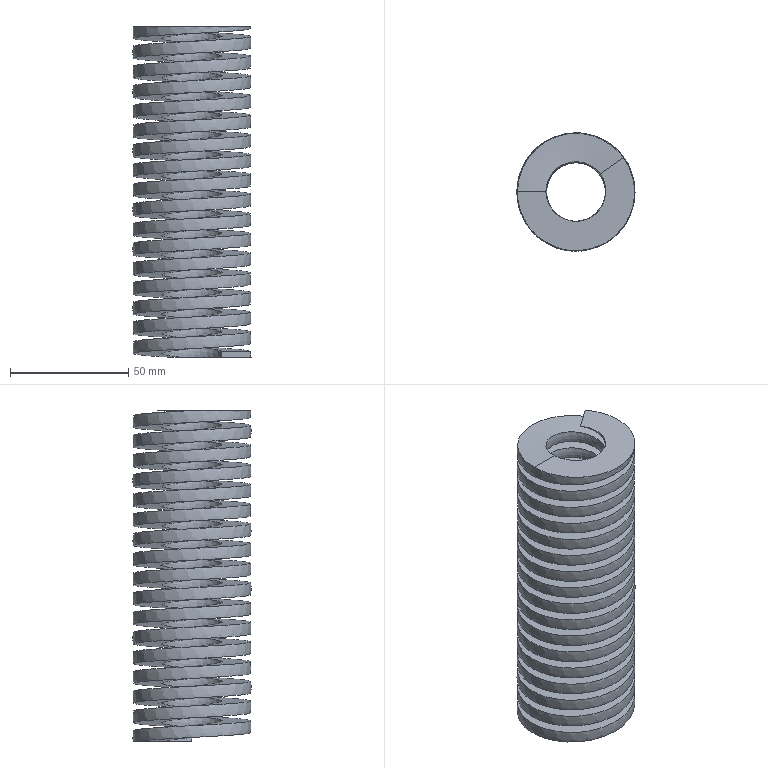Part | Creo | 1 solid | 7 faces | box 50.006 x 50.005 x 140.001 mm | volume 124778 mm3 | spline 4 | plane 3